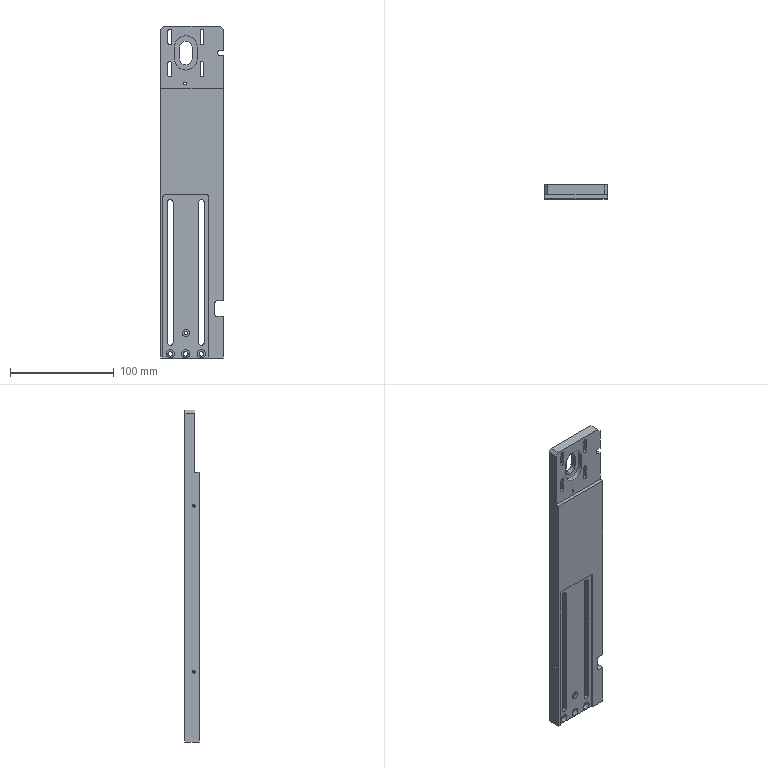Part | NX | features BREP 1 | 1 solid | 189 faces | box 60 x 13.5 x 320 mm | volume 187245 mm3 | cylinder 98 | plane 71 | cone 20 | commonest cylinder face diameters 2.5 x24 3.4 x14 6 x12 4 x10 3 x6 4.5 x6